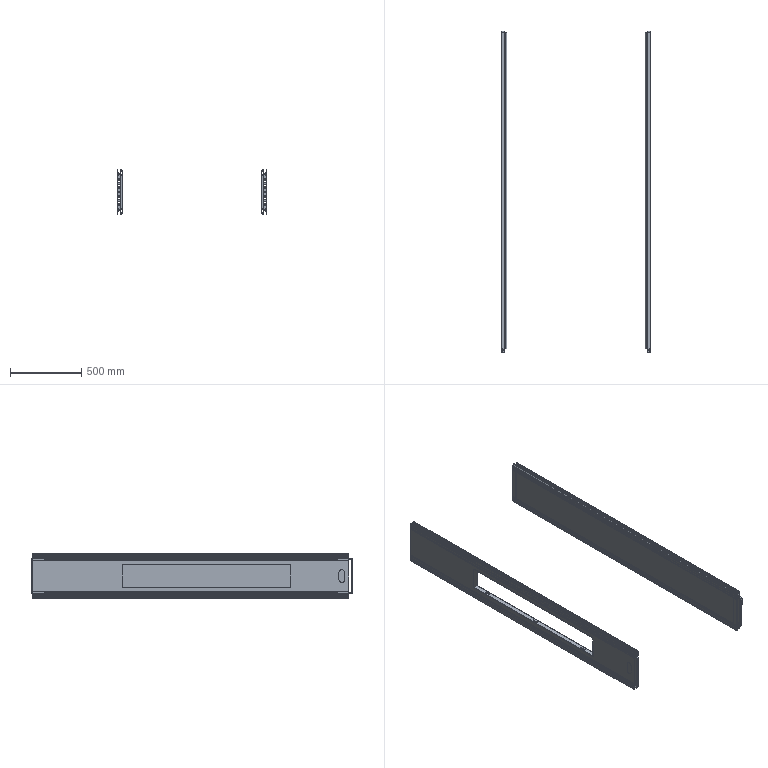Part | SolidWorks | features ReferencePattern 11, MirrorCompFeat 3 | 50 solids | 1380 faces | box 1050 x 2251 x 320 mm | volume 8474214 mm3 | plane 828 | cylinder 552 | commonest cylinder face diameters 8.5 x80 8 x74 6 x72 6.2 x48 8.2 x48 12 x48